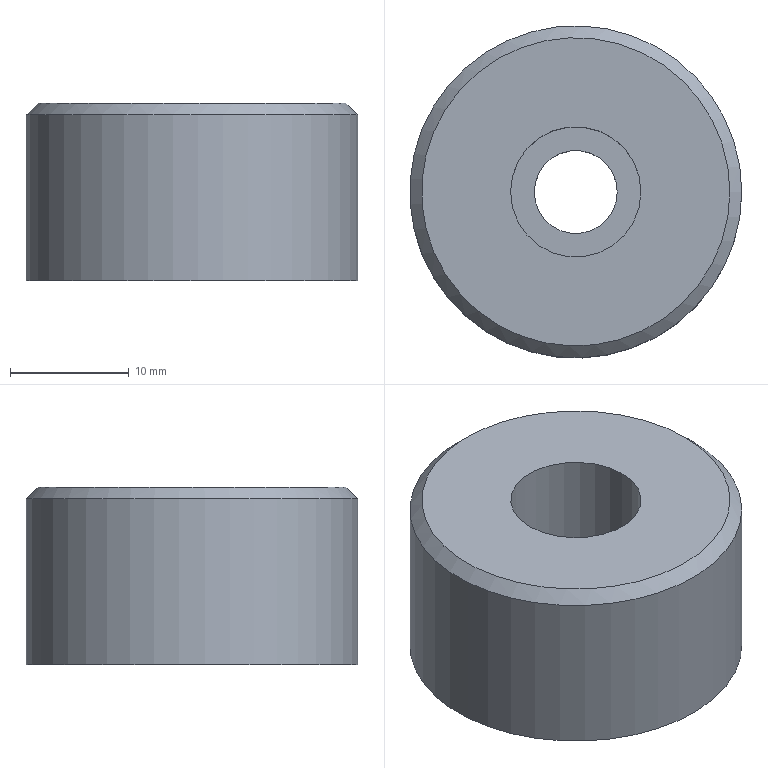Part | NX | features 21 2 | 1 solid | 7 faces | box 28 x 28 x 15 mm | volume 8164 mm3 | cylinder 3 | plane 3 | cone 1 | commonest cylinder face diameters 7 x1 11 x1 28 x1
STEP:
#1=CARTESIAN_POINT('',(3109.,440.,-1.1));
#2=VERTEX_POINT('',#1);
#3=CARTESIAN_POINT('',(3095.,440.,-1.1));
#4=DIRECTION('',(0.,0.,1.));
#5=DIRECTION('',(1.,0.,0.));
#6=AXIS2_PLACEMENT_3D('',#3,#4,#5);
#7=CIRCLE('',#6,14.);
#8=EDGE_CURVE('',#2,#2,#7,.T.);
#9=ORIENTED_EDGE('',*,*,#8,.F.);
#10=EDGE_LOOP('',(#9));
#11=FACE_BOUND('',#10,.T.);
#12=CARTESIAN_POINT('',(3109.,440.,-15.1));
#13=VERTEX_POINT('',#12);
#14=CARTESIAN_POINT('',(3095.,440.,-15.1));
#15=DIRECTION('',(0.,0.,-1.));
#16=DIRECTION('',(1.,0.,0.));
#17=AXIS2_PLACEMENT_3D('',#14,#15,#16);
#18=CIRCLE('',#17,14.);
#19=EDGE_CURVE('',#13,#13,#18,.T.);
#20=ORIENTED_EDGE('',*,*,#19,.F.);
#21=EDGE_LOOP('',(#20));
#22=FACE_BOUND('',#21,.T.);
#23=CARTESIAN_POINT('',(3095.,440.,-7.1));
#24=DIRECTION('',(0.,0.,-1.));
#25=DIRECTION('',(-1.,0.,0.));
#26=AXIS2_PLACEMENT_3D('',#23,#24,#25);
#27=CYLINDRICAL_SURFACE('',#26,14.);
#28=ADVANCED_FACE('',(#11,#22),#27,.T.);
#29=CARTESIAN_POINT('',(3108.,440.,-0.1));
#30=VERTEX_POINT('',#29);
#31=CARTESIAN_POINT('',(3095.,440.,-0.1));
#32=DIRECTION('',(0.,0.,-1.));
#33=DIRECTION('',(1.,0.,0.));
#34=AXIS2_PLACEMENT_3D('',#31,#32,#33);
#35=CIRCLE('',#34,13.);
#36=EDGE_CURVE('',#30,#30,#35,.T.);
#37=ORIENTED_EDGE('',*,*,#36,.F.);
#38=EDGE_LOOP('',(#37));
#39=FACE_BOUND('',#38,.T.);
#40=CARTESIAN_POINT('',(3100.5,440.,-0.1));
#41=VERTEX_POINT('',#40);
#42=CARTESIAN_POINT('',(3095.,440.,-0.1));
#43=DIRECTION('',(0.,0.,1.));
#44=DIRECTION('',(1.,0.,0.));
#45=AXIS2_PLACEMENT_3D('',#42,#43,#44);
#46=CIRCLE('',#45,5.5);
#47=EDGE_CURVE('',#41,#41,#46,.T.);
#48=ORIENTED_EDGE('',*,*,#47,.F.);
#49=EDGE_LOOP('',(#48));
#50=FACE_BOUND('',#49,.T.);
#51=CARTESIAN_POINT('',(3095.,440.,-0.1));
#52=DIRECTION('',(0.,0.,1.));
#53=DIRECTION('',(1.,0.,0.));
#54=AXIS2_PLACEMENT_3D('',#51,#52,#53);
#55=PLANE('',#54);
#56=ADVANCED_FACE('',(#39,#50),#55,.T.);
#57=ORIENTED_EDGE('',*,*,#19,.T.);
#58=EDGE_LOOP('',(#57));
#59=FACE_BOUND('',#58,.T.);
#60=CARTESIAN_POINT('',(3098.5,440.,-15.1));
#61=VERTEX_POINT('',#60);
#62=CARTESIAN_POINT('',(3095.,440.,-15.1));
#63=DIRECTION('',(0.,0.,-1.));
#64=DIRECTION('',(1.,0.,0.));
#65=AXIS2_PLACEMENT_3D('',#62,#63,#64);
#66=CIRCLE('',#65,3.5);
#67=EDGE_CURVE('',#61,#61,#66,.T.);
#68=ORIENTED_EDGE('',*,*,#67,.F.);
#69=EDGE_LOOP('',(#68));
#70=FACE_BOUND('',#69,.T.);
#71=CARTESIAN_POINT('',(2992.879,-62.728,-15.1));
#72=DIRECTION('',(0.,0.,1.));
#73=DIRECTION('',(1.,0.,0.));
#74=AXIS2_PLACEMENT_3D('',#71,#72,#73);
#75=PLANE('',#74);
#76=ADVANCED_FACE('',(#59,#70),#75,.F.);
#77=ORIENTED_EDGE('',*,*,#47,.T.);
#78=EDGE_LOOP('',(#77));
#79=FACE_BOUND('',#78,.T.);
#80=CARTESIAN_POINT('',(3089.5,440.,-8.1));
#81=VERTEX_POINT('',#80);
#82=CARTESIAN_POINT('',(3095.,440.,-8.1));
#83=DIRECTION('',(0.,0.,1.));
#84=DIRECTION('',(-1.,0.,0.));
#85=AXIS2_PLACEMENT_3D('',#82,#83,#84);
#86=CIRCLE('',#85,5.5);
#87=EDGE_CURVE('',#81,#81,#86,.T.);
#88=ORIENTED_EDGE('',*,*,#87,.F.);
#89=EDGE_LOOP('',(#88));
#90=FACE_BOUND('',#89,.T.);
#91=CARTESIAN_POINT('',(3095.,440.,-15.1));
#92=DIRECTION('',(0.,0.,1.));
#93=DIRECTION('',(1.,0.,0.));
#94=AXIS2_PLACEMENT_3D('',#91,#92,#93);
#95=CYLINDRICAL_SURFACE('',#94,5.5);
#96=ADVANCED_FACE('',(#79,#90),#95,.F.);
#97=CARTESIAN_POINT('',(3091.5,440.,-8.1));
#98=VERTEX_POINT('',#97);
#99=CARTESIAN_POINT('',(3095.,440.,-8.1));
#100=DIRECTION('',(0.,0.,1.));
#101=DIRECTION('',(-1.,0.,0.));
#102=AXIS2_PLACEMENT_3D('',#99,#100,#101);
#103=CIRCLE('',#102,3.5);
#104=EDGE_CURVE('',#98,#98,#103,.T.);
#105=ORIENTED_EDGE('',*,*,#104,.T.);
#106=EDGE_LOOP('',(#105));
#107=FACE_BOUND('',#106,.T.);
#108=ORIENTED_EDGE('',*,*,#67,.T.);
#109=EDGE_LOOP('',(#108));
#110=FACE_BOUND('',#109,.T.);
#111=CARTESIAN_POINT('',(3095.,440.,-7.1));
#112=DIRECTION('',(0.,0.,-1.));
#113=DIRECTION('',(-1.,0.,0.));
#114=AXIS2_PLACEMENT_3D('',#111,#112,#113);
#115=CYLINDRICAL_SURFACE('',#114,3.5);
#116=ADVANCED_FACE('',(#107,#110),#115,.F.);
#117=ORIENTED_EDGE('',*,*,#104,.F.);
#118=EDGE_LOOP('',(#117));
#119=FACE_BOUND('',#118,.T.);
#120=ORIENTED_EDGE('',*,*,#87,.T.);
#121=EDGE_LOOP('',(#120));
#122=FACE_BOUND('',#121,.T.);
#123=CARTESIAN_POINT('',(3095.,440.,-8.1));
#124=DIRECTION('',(0.,0.,-1.));
#125=DIRECTION('',(-1.,0.,0.));
#126=AXIS2_PLACEMENT_3D('',#123,#124,#125);
#127=PLANE('',#126);
#128=ADVANCED_FACE('',(#119,#122),#127,.F.);
#129=ORIENTED_EDGE('',*,*,#36,.T.);
#130=EDGE_LOOP('',(#129));
#131=FACE_BOUND('',#130,.T.);
#132=ORIENTED_EDGE('',*,*,#8,.T.);
#133=EDGE_LOOP('',(#132));
#134=FACE_BOUND('',#133,.T.);
#135=CARTESIAN_POINT('',(3095.,440.,-1.1));
#136=DIRECTION('',(0.,0.,-1.));
#137=DIRECTION('',(1.,0.,0.));
#138=AXIS2_PLACEMENT_3D('',#135,#136,#137);
#139=CONICAL_SURFACE('',#138,14.,0.7854);
#140=ADVANCED_FACE('',(#131,#134),#139,.T.);
#141=CLOSED_SHELL('',(#28,#56,#76,#96,#116,#128,#140));
#142=MANIFOLD_SOLID_BREP('',#141);
#143=(LENGTH_UNIT()NAMED_UNIT(*)SI_UNIT(.MILLI.,.METRE.));
#144=UNCERTAINTY_MEASURE_WITH_UNIT(LENGTH_MEASURE(0.00001),#143,'','');
#145=(NAMED_UNIT(*)PLANE_ANGLE_UNIT()SI_UNIT($,.RADIAN.));
#146=(NAMED_UNIT(*)SI_UNIT($,.STERADIAN.)SOLID_ANGLE_UNIT());
#147=(GEOMETRIC_REPRESENTATION_CONTEXT(3)GLOBAL_UNCERTAINTY_ASSIGNED_CONTEXT((#144))GLOBAL_UNIT_ASSIGNED_CONTEXT((#143,#145,#146))REPRESENTATION_CONTEXT('',''));
#148=ADVANCED_BREP_SHAPE_REPRESENTATION('',(#142),#147);